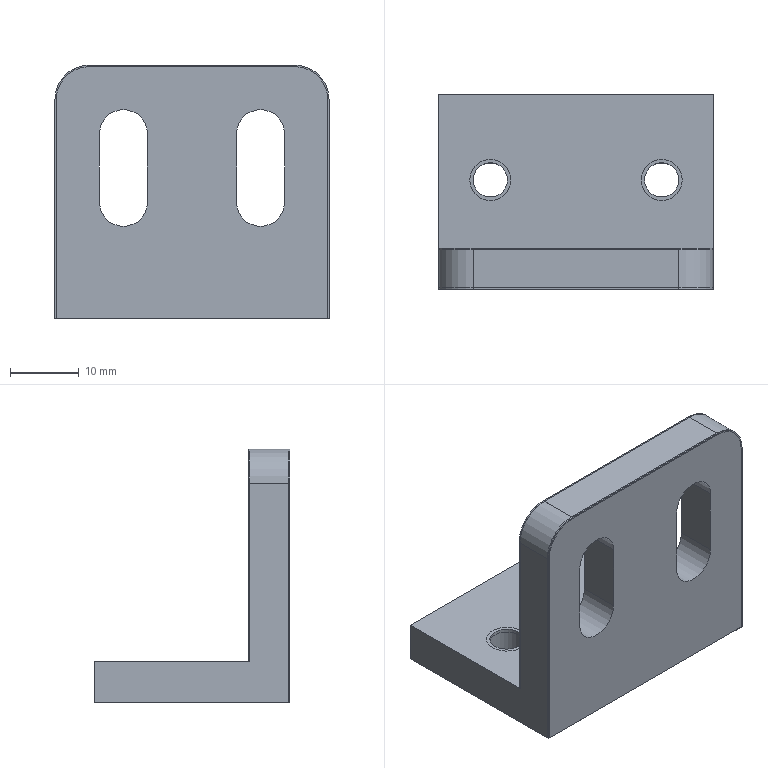NC program | NX | posted with a generic post | part box 40 x 28.5 x 37 mm
Lines 1289 to 1837 of 1837:
(CURVE_DRIVE_COPY_2 , TOOL : SPHERICAL_MILL)
N2564 T20 M6
N2566 G53
N2568 G17 G0 G90 X12.364 Y-15.864 B0. C0. S3500 M3
N2570 G43 Z50. H20
N2572 Z-15.5 B-180.
N2574 G94 G1 X8.121 Y-11.621 F60.
N2576 Y-11.622 Z-15.457
N2578 Y-11.626 Z-15.414
N2580 Y-11.631 Z-15.371
N2582 Y-11.638 Z-15.329
N2584 Y-11.648 Z-15.286
N2586 Y-11.659 Z-15.245
N2588 Y-11.673 Z-15.204
N2590 Y-11.688 Z-15.164
N2592 Y-11.706 Z-15.124
N2594 Y-11.725 Z-15.086
N2596 Y-11.746 Z-15.048
N2598 Y-11.769 Z-15.012
N2600 Y-11.794 Z-14.977
N2602 Y-11.821 Z-14.943
N2604 Y-11.849 Z-14.91
N2606 Y-11.879 Z-14.879
N2608 Y-11.91 Z-14.849
N2610 Y-11.943 Z-14.821
N2612 Y-11.977 Z-14.794
N2614 Y-12.012 Z-14.769
N2616 Y-12.048 Z-14.746
N2618 Y-12.086 Z-14.725
N2620 Y-12.124 Z-14.706
N2622 Y-12.164 Z-14.688
N2624 Y-12.204 Z-14.673
N2626 Y-12.245 Z-14.659
N2628 Y-12.286 Z-14.648
N2630 Y-12.329 Z-14.638
N2632 Y-12.371 Z-14.631
N2634 Y-12.414 Z-14.626
N2636 Y-12.457 Z-14.622
N2638 Y-12.5 Z-14.621
N2640 Y-12.543 Z-14.622
N2642 Y-12.586 Z-14.626
N2644 Y-12.629 Z-14.631
N2646 Y-12.671 Z-14.638
N2648 Y-12.714 Z-14.648
N2650 Y-12.755 Z-14.659
N2652 Y-12.796 Z-14.673
N2654 Y-12.836 Z-14.688
N2656 Y-12.876 Z-14.706
N2658 Y-12.914 Z-14.725
N2660 Y-12.952 Z-14.746
N2662 Y-12.988 Z-14.769
N2664 Y-13.023 Z-14.794
N2666 Y-13.057 Z-14.821
N2668 Y-13.09 Z-14.849
N2670 Y-13.121 Z-14.879
N2672 Y-13.151 Z-14.91
N2674 Y-13.179 Z-14.943
N2676 Y-13.206 Z-14.977
N2678 Y-13.231 Z-15.012
N2680 Y-13.254 Z-15.048
N2682 Y-13.275 Z-15.086
N2684 Y-13.294 Z-15.124
N2686 Y-13.312 Z-15.164
N2688 Y-13.327 Z-15.204
N2690 Y-13.341 Z-15.245
N2692 Y-13.352 Z-15.286
N2694 Y-13.362 Z-15.329
N2696 Y-13.369 Z-15.371
N2698 Y-13.374 Z-15.414
N2700 Y-13.378 Z-15.457
N2702 Y-13.379 Z-15.5
N2704 Y-13.378 Z-15.543
N2706 Y-13.374 Z-15.586
N2708 Y-13.369 Z-15.629
N2710 Y-13.362 Z-15.671
N2712 Y-13.352 Z-15.714
N2714 Y-13.341 Z-15.755
N2716 Y-13.327 Z-15.796
N2718 Y-13.312 Z-15.836
N2720 Y-13.294 Z-15.876
N2722 Y-13.275 Z-15.914
N2724 Y-13.254 Z-15.952
N2726 Y-13.231 Z-15.988
N2728 Y-13.206 Z-16.023
N2730 Y-13.179 Z-16.057
N2732 Y-13.151 Z-16.09
N2734 Y-13.121 Z-16.121
N2736 Y-13.09 Z-16.151
N2738 Y-13.057 Z-16.179
N2740 Y-13.023 Z-16.206
N2742 Y-12.988 Z-16.231
N2744 Y-12.952 Z-16.254
N2746 Y-12.914 Z-16.275
N2748 Y-12.876 Z-16.294
N2750 Y-12.836 Z-16.312
N2752 Y-12.796 Z-16.327
N2754 Y-12.755 Z-16.341
N2756 Y-12.714 Z-16.352
N2758 Y-12.671 Z-16.362
N2760 Y-12.629 Z-16.369
N2762 Y-12.586 Z-16.374
N2764 Y-12.543 Z-16.378
N2766 Y-12.5 Z-16.379
N2768 Y-12.457 Z-16.378
N2770 Y-12.414 Z-16.374
N2772 Y-12.371 Z-16.369
N2774 Y-12.329 Z-16.362
N2776 Y-12.286 Z-16.352
N2778 Y-12.245 Z-16.341
N2780 Y-12.204 Z-16.327
N2782 Y-12.164 Z-16.312
N2784 Y-12.124 Z-16.294
N2786 Y-12.086 Z-16.275
N2788 Y-12.048 Z-16.254
N2790 Y-12.012 Z-16.231
N2792 Y-11.977 Z-16.206
N2794 Y-11.943 Z-16.179
N2796 Y-11.91 Z-16.151
N2798 Y-11.879 Z-16.121
N2800 Y-11.849 Z-16.09
N2802 Y-11.821 Z-16.057
N2804 Y-11.794 Z-16.023
N2806 Y-11.769 Z-15.988
N2808 Y-11.746 Z-15.952
N2810 Y-11.725 Z-15.914
N2812 Y-11.706 Z-15.876
N2814 Y-11.688 Z-15.836
N2816 Y-11.673 Z-15.796
N2818 Y-11.659 Z-15.755
N2820 Y-11.648 Z-15.714
N2822 Y-11.638 Z-15.671
N2824 Y-11.631 Z-15.629
N2826 Y-11.626 Z-15.586
N2828 Y-11.622 Z-15.543
N2830 Y-11.621 Z-15.5
N2832 X12.364 Y-15.864
N2834 G0 Z50.
(CURVE_DRIVE_COPY_COPY , TOOL : SPHERICAL_MILL)
N2836 Y9.136
N2838 Z-15.5
N2840 G1 X8.121 Y13.379
N2842 Y13.378 Z-15.457
N2844 Y13.374 Z-15.414
N2846 Y13.369 Z-15.371
N2848 Y13.362 Z-15.329
N2850 Y13.352 Z-15.286
N2852 Y13.341 Z-15.245
N2854 Y13.327 Z-15.204
N2856 Y13.312 Z-15.164
N2858 Y13.294 Z-15.124
N2860 Y13.275 Z-15.086
N2862 Y13.254 Z-15.048
N2864 Y13.231 Z-15.012
N2866 Y13.206 Z-14.977
N2868 Y13.179 Z-14.943
N2870 Y13.151 Z-14.91
N2872 Y13.121 Z-14.879
N2874 Y13.09 Z-14.849
N2876 Y13.057 Z-14.821
N2878 Y13.023 Z-14.794
N2880 Y12.988 Z-14.769
N2882 Y12.952 Z-14.746
N2884 Y12.914 Z-14.725
N2886 Y12.876 Z-14.706
N2888 Y12.836 Z-14.688
N2890 Y12.796 Z-14.673
N2892 Y12.755 Z-14.659
N2894 Y12.714 Z-14.648
N2896 Y12.671 Z-14.638
N2898 Y12.629 Z-14.631
N2900 Y12.586 Z-14.626
N2902 Y12.543 Z-14.622
N2904 Y12.5 Z-14.621
N2906 Y12.457 Z-14.622
N2908 Y12.414 Z-14.626
N2910 Y12.371 Z-14.631
N2912 Y12.329 Z-14.638
N2914 Y12.286 Z-14.648
N2916 Y12.245 Z-14.659
N2918 Y12.204 Z-14.673
N2920 Y12.164 Z-14.688
N2922 Y12.124 Z-14.706
N2924 Y12.086 Z-14.725
N2926 Y12.048 Z-14.746
N2928 Y12.012 Z-14.769
N2930 Y11.977 Z-14.794
N2932 Y11.943 Z-14.821
N2934 Y11.91 Z-14.849
N2936 Y11.879 Z-14.879
N2938 Y11.849 Z-14.91
N2940 Y11.821 Z-14.943
N2942 Y11.794 Z-14.977
N2944 Y11.769 Z-15.012
N2946 Y11.746 Z-15.048
N2948 Y11.725 Z-15.086
N2950 Y11.706 Z-15.124
N2952 Y11.688 Z-15.164
N2954 Y11.673 Z-15.204
N2956 Y11.659 Z-15.245
N2958 Y11.648 Z-15.286
N2960 Y11.638 Z-15.329
N2962 Y11.631 Z-15.371
N2964 Y11.626 Z-15.414
N2966 Y11.622 Z-15.457
N2968 Y11.621 Z-15.5
N2970 Y11.622 Z-15.543
N2972 Y11.626 Z-15.586
N2974 Y11.631 Z-15.629
N2976 Y11.638 Z-15.671
N2978 Y11.648 Z-15.714
N2980 Y11.659 Z-15.755
N2982 Y11.673 Z-15.796
N2984 Y11.688 Z-15.836
N2986 Y11.706 Z-15.876
N2988 Y11.725 Z-15.914
N2990 Y11.746 Z-15.952
N2992 Y11.769 Z-15.988
N2994 Y11.794 Z-16.023
N2996 Y11.821 Z-16.057
N2998 Y11.849 Z-16.09
N3000 Y11.879 Z-16.121
N3002 Y11.91 Z-16.151
N3004 Y11.943 Z-16.179
N3006 Y11.977 Z-16.206
N3008 Y12.012 Z-16.231
N3010 Y12.048 Z-16.254
N3012 Y12.086 Z-16.275
N3014 Y12.124 Z-16.294
N3016 Y12.164 Z-16.312
N3018 Y12.204 Z-16.327
N3020 Y12.245 Z-16.341
N3022 Y12.286 Z-16.352
N3024 Y12.329 Z-16.362
N3026 Y12.371 Z-16.369
N3028 Y12.414 Z-16.374
N3030 Y12.457 Z-16.378
N3032 Y12.5 Z-16.379
N3034 Y12.543 Z-16.378
N3036 Y12.586 Z-16.374
N3038 Y12.629 Z-16.369
N3040 Y12.671 Z-16.362
N3042 Y12.714 Z-16.352
N3044 Y12.755 Z-16.341
N3046 Y12.796 Z-16.327
N3048 Y12.836 Z-16.312
N3050 Y12.876 Z-16.294
N3052 Y12.914 Z-16.275
N3054 Y12.952 Z-16.254
N3056 Y12.988 Z-16.231
N3058 Y13.023 Z-16.206
N3060 Y13.057 Z-16.179
N3062 Y13.09 Z-16.151
N3064 Y13.121 Z-16.121
N3066 Y13.151 Z-16.09
N3068 Y13.179 Z-16.057
N3070 Y13.206 Z-16.023
N3072 Y13.231 Z-15.988
N3074 Y13.254 Z-15.952
N3076 Y13.275 Z-15.914
N3078 Y13.294 Z-15.876
N3080 Y13.312 Z-15.836
N3082 Y13.327 Z-15.796
N3084 Y13.341 Z-15.755
N3086 Y13.352 Z-15.714
N3088 Y13.362 Z-15.671
N3090 Y13.369 Z-15.629
N3092 Y13.374 Z-15.586
N3094 Y13.378 Z-15.543
N3096 Y13.379 Z-15.5
N3098 X12.364 Y9.136
N3100 G0 Z50.
(CURVE_DRIVE_COPY_2_COPY , TOOL : SPHERICAL_MILL)
N3102 X12.35 Y-15.85
N3104 Z-15.5
N3106 G1 X8.107 Y-11.607
N3108 Y-11.608 Z-15.544
N3110 Y-11.611 Z-15.588
N3112 Y-11.617 Z-15.631
N3114 Y-11.624 Z-15.674
N3116 Y-11.634 Z-15.717
N3118 Y-11.646 Z-15.759
N3120 Y-11.659 Z-15.801
N3122 Y-11.675 Z-15.842
N3124 Y-11.693 Z-15.882
N3126 Y-11.713 Z-15.921
N3128 Y-11.734 Z-15.959
N3130 Y-11.758 Z-15.996
N3132 Y-11.783 Z-16.032
N3134 Y-11.81 Z-16.066
N3136 Y-11.838 Z-16.1
N3138 Y-11.869 Z-16.131
N3140 Y-11.9 Z-16.162
N3142 Y-11.934 Z-16.19
N3144 Y-11.968 Z-16.217
N3146 Y-12.004 Z-16.242
N3148 Y-12.041 Z-16.266
N3150 Y-12.079 Z-16.287
N3152 Y-12.118 Z-16.307
N3154 Y-12.158 Z-16.325
N3156 Y-12.199 Z-16.341
N3158 Y-12.241 Z-16.354
N3160 Y-12.283 Z-16.366
N3162 Y-12.326 Z-16.376
N3164 Y-12.369 Z-16.383
N3166 Y-12.412 Z-16.389
N3168 Y-12.456 Z-16.392
N3170 Y-12.5 Z-16.393
N3172 Y-12.544 Z-16.392
N3174 Y-12.588 Z-16.389
N3176 Y-12.631 Z-16.383
N3178 Y-12.674 Z-16.376
N3180 Y-12.717 Z-16.366
N3182 Y-12.759 Z-16.354
N3184 Y-12.801 Z-16.341
N3186 Y-12.842 Z-16.325
N3188 Y-12.882 Z-16.307
N3190 Y-12.921 Z-16.287
N3192 Y-12.959 Z-16.266
N3194 Y-12.996 Z-16.242
N3196 Y-13.032 Z-16.217
N3198 Y-13.066 Z-16.19
N3200 Y-13.1 Z-16.162
N3202 Y-13.131 Z-16.131
N3204 Y-13.162 Z-16.1
N3206 Y-13.19 Z-16.066
N3208 Y-13.217 Z-16.032
N3210 Y-13.242 Z-15.996
N3212 Y-13.266 Z-15.959
N3214 Y-13.287 Z-15.921
N3216 Y-13.307 Z-15.882
N3218 Y-13.325 Z-15.842
N3220 Y-13.341 Z-15.801
N3222 Y-13.354 Z-15.759
N3224 Y-13.366 Z-15.717
N3226 Y-13.376 Z-15.674
N3228 Y-13.383 Z-15.631
N3230 Y-13.389 Z-15.588
N3232 Y-13.392 Z-15.544
N3234 Y-13.393 Z-15.5
N3236 Y-13.392 Z-15.456
N3238 Y-13.389 Z-15.412
N3240 Y-13.383 Z-15.369
N3242 Y-13.376 Z-15.326
N3244 Y-13.366 Z-15.283
N3246 Y-13.354 Z-15.241
N3248 Y-13.341 Z-15.199
N3250 Y-13.325 Z-15.158
N3252 Y-13.307 Z-15.118
N3254 Y-13.287 Z-15.079
N3256 Y-13.266 Z-15.041
N3258 Y-13.242 Z-15.004
N3260 Y-13.217 Z-14.968
N3262 Y-13.19 Z-14.934
N3264 Y-13.162 Z-14.9
N3266 Y-13.131 Z-14.869
N3268 Y-13.1 Z-14.838
N3270 Y-13.066 Z-14.81
N3272 Y-13.032 Z-14.783
N3274 Y-12.996 Z-14.758
N3276 Y-12.959 Z-14.734
N3278 Y-12.921 Z-14.713
N3280 Y-12.882 Z-14.693
N3282 Y-12.842 Z-14.675
N3284 Y-12.801 Z-14.659
N3286 Y-12.759 Z-14.646
N3288 Y-12.717 Z-14.634
N3290 Y-12.674 Z-14.624
N3292 Y-12.631 Z-14.617
N3294 Y-12.588 Z-14.611
N3296 Y-12.544 Z-14.608
N3298 Y-12.5 Z-14.607
N3300 Y-12.456 Z-14.608
N3302 Y-12.412 Z-14.611
N3304 Y-12.369 Z-14.617
N3306 Y-12.326 Z-14.624
N3308 Y-12.283 Z-14.634
N3310 Y-12.241 Z-14.646
N3312 Y-12.199 Z-14.659
N3314 Y-12.158 Z-14.675
N3316 Y-12.118 Z-14.693
N3318 Y-12.079 Z-14.713
N3320 Y-12.041 Z-14.734
N3322 Y-12.004 Z-14.758
N3324 Y-11.968 Z-14.783
N3326 Y-11.934 Z-14.81
N3328 Y-11.9 Z-14.838
N3330 Y-11.869 Z-14.869
N3332 Y-11.838 Z-14.9
N3334 Y-11.81 Z-14.934
N3336 Y-11.783 Z-14.968
N3338 Y-11.758 Z-15.004
N3340 Y-11.734 Z-15.041
N3342 Y-11.713 Z-15.079
N3344 Y-11.693 Z-15.118
N3346 Y-11.675 Z-15.158
N3348 Y-11.659 Z-15.199
N3350 Y-11.646 Z-15.241
N3352 Y-11.634 Z-15.283
N3354 Y-11.624 Z-15.326
N3356 Y-11.617 Z-15.369
N3358 Y-11.611 Z-15.412
N3360 Y-11.608 Z-15.456
N3362 Y-11.607 Z-15.5
N3364 X12.35 Y-15.85
N3366 G0 Z50.
(CURVE_DRIVE_COPY_COPY_COPY , TOOL : SPHERICAL_MILL)
N3368 Y9.15
N3370 Z-15.5
N3372 G1 X8.107 Y13.393
N3374 Y13.392 Z-15.544
N3376 Y13.389 Z-15.588
N3378 Y13.383 Z-15.631
N3380 Y13.376 Z-15.674
N3382 Y13.366 Z-15.717
N3384 Y13.354 Z-15.759
N3386 Y13.341 Z-15.801
N3388 Y13.325 Z-15.842
N3390 Y13.307 Z-15.882
N3392 Y13.287 Z-15.921
N3394 Y13.266 Z-15.959
N3396 Y13.242 Z-15.996
N3398 Y13.217 Z-16.032
N3400 Y13.19 Z-16.066
N3402 Y13.162 Z-16.1
N3404 Y13.131 Z-16.131
N3406 Y13.1 Z-16.162
N3408 Y13.066 Z-16.19
N3410 Y13.032 Z-16.217
N3412 Y12.996 Z-16.242
N3414 Y12.959 Z-16.266
N3416 Y12.921 Z-16.287
N3418 Y12.882 Z-16.307
N3420 Y12.842 Z-16.325
N3422 Y12.801 Z-16.341
N3424 Y12.759 Z-16.354
N3426 Y12.717 Z-16.366
N3428 Y12.674 Z-16.376
N3430 Y12.631 Z-16.383
N3432 Y12.588 Z-16.389
N3434 Y12.544 Z-16.392
N3436 Y12.5 Z-16.393
N3438 Y12.456 Z-16.392
N3440 Y12.412 Z-16.389
N3442 Y12.369 Z-16.383
N3444 Y12.326 Z-16.376
N3446 Y12.283 Z-16.366
N3448 Y12.241 Z-16.354
N3450 Y12.199 Z-16.341
N3452 Y12.158 Z-16.325
N3454 Y12.118 Z-16.307
N3456 Y12.079 Z-16.287
N3458 Y12.041 Z-16.266
N3460 Y12.004 Z-16.242
N3462 Y11.968 Z-16.217
N3464 Y11.934 Z-16.19
N3466 Y11.9 Z-16.162
N3468 Y11.869 Z-16.131
N3470 Y11.838 Z-16.1
N3472 Y11.81 Z-16.066
N3474 Y11.783 Z-16.032
N3476 Y11.758 Z-15.996
N3478 Y11.734 Z-15.959
N3480 Y11.713 Z-15.921
N3482 Y11.693 Z-15.882
N3484 Y11.675 Z-15.842
N3486 Y11.659 Z-15.801
N3488 Y11.646 Z-15.759
N3490 Y11.634 Z-15.717
N3492 Y11.624 Z-15.674
N3494 Y11.617 Z-15.631
N3496 Y11.611 Z-15.588
N3498 Y11.608 Z-15.544
N3500 Y11.607 Z-15.5
N3502 Y11.608 Z-15.456
N3504 Y11.611 Z-15.412
N3506 Y11.617 Z-15.369
N3508 Y11.624 Z-15.326
N3510 Y11.634 Z-15.283
N3512 Y11.646 Z-15.241
N3514 Y11.659 Z-15.199
N3516 Y11.675 Z-15.158
N3518 Y11.693 Z-15.118
N3520 Y11.713 Z-15.079
N3522 Y11.734 Z-15.041
N3524 Y11.758 Z-15.004
N3526 Y11.783 Z-14.968
N3528 Y11.81 Z-14.934
N3530 Y11.838 Z-14.9
N3532 Y11.869 Z-14.869
N3534 Y11.9 Z-14.838
N3536 Y11.934 Z-14.81
N3538 Y11.968 Z-14.783
N3540 Y12.004 Z-14.758
N3542 Y12.041 Z-14.734
N3544 Y12.079 Z-14.713
N3546 Y12.118 Z-14.693
N3548 Y12.158 Z-14.675
N3550 Y12.199 Z-14.659
N3552 Y12.241 Z-14.646
N3554 Y12.283 Z-14.634
N3556 Y12.326 Z-14.624
N3558 Y12.369 Z-14.617
N3560 Y12.412 Z-14.611
N3562 Y12.456 Z-14.608
N3564 Y12.5 Z-14.607
N3566 Y12.544 Z-14.608
N3568 Y12.588 Z-14.611
N3570 Y12.631 Z-14.617
N3572 Y12.674 Z-14.624
N3574 Y12.717 Z-14.634
N3576 Y12.759 Z-14.646
N3578 Y12.801 Z-14.659
N3580 Y12.842 Z-14.675
N3582 Y12.882 Z-14.693
N3584 Y12.921 Z-14.713
N3586 Y12.959 Z-14.734
N3588 Y12.996 Z-14.758
N3590 Y13.032 Z-14.783
N3592 Y13.066 Z-14.81
N3594 Y13.1 Z-14.838
N3596 Y13.131 Z-14.869
N3598 Y13.162 Z-14.9
N3600 Y13.19 Z-14.934
N3602 Y13.217 Z-14.968
N3604 Y13.242 Z-15.004
N3606 Y13.266 Z-15.041
N3608 Y13.287 Z-15.079
N3610 Y13.307 Z-15.118
N3612 Y13.325 Z-15.158
N3614 Y13.341 Z-15.199
N3616 Y13.354 Z-15.241
N3618 Y13.366 Z-15.283
N3620 Y13.376 Z-15.326
N3622 Y13.383 Z-15.369
N3624 Y13.389 Z-15.412
N3626 Y13.392 Z-15.456
N3628 Y13.393 Z-15.5
N3630 X12.35 Y9.15
N3632 G0 Z50.
N3634 M5
N3636 M2